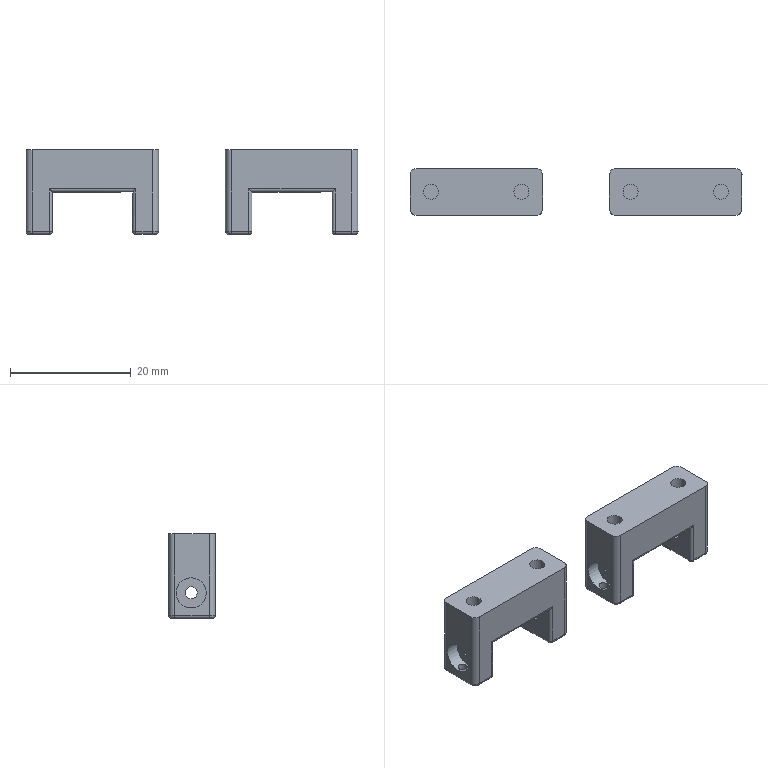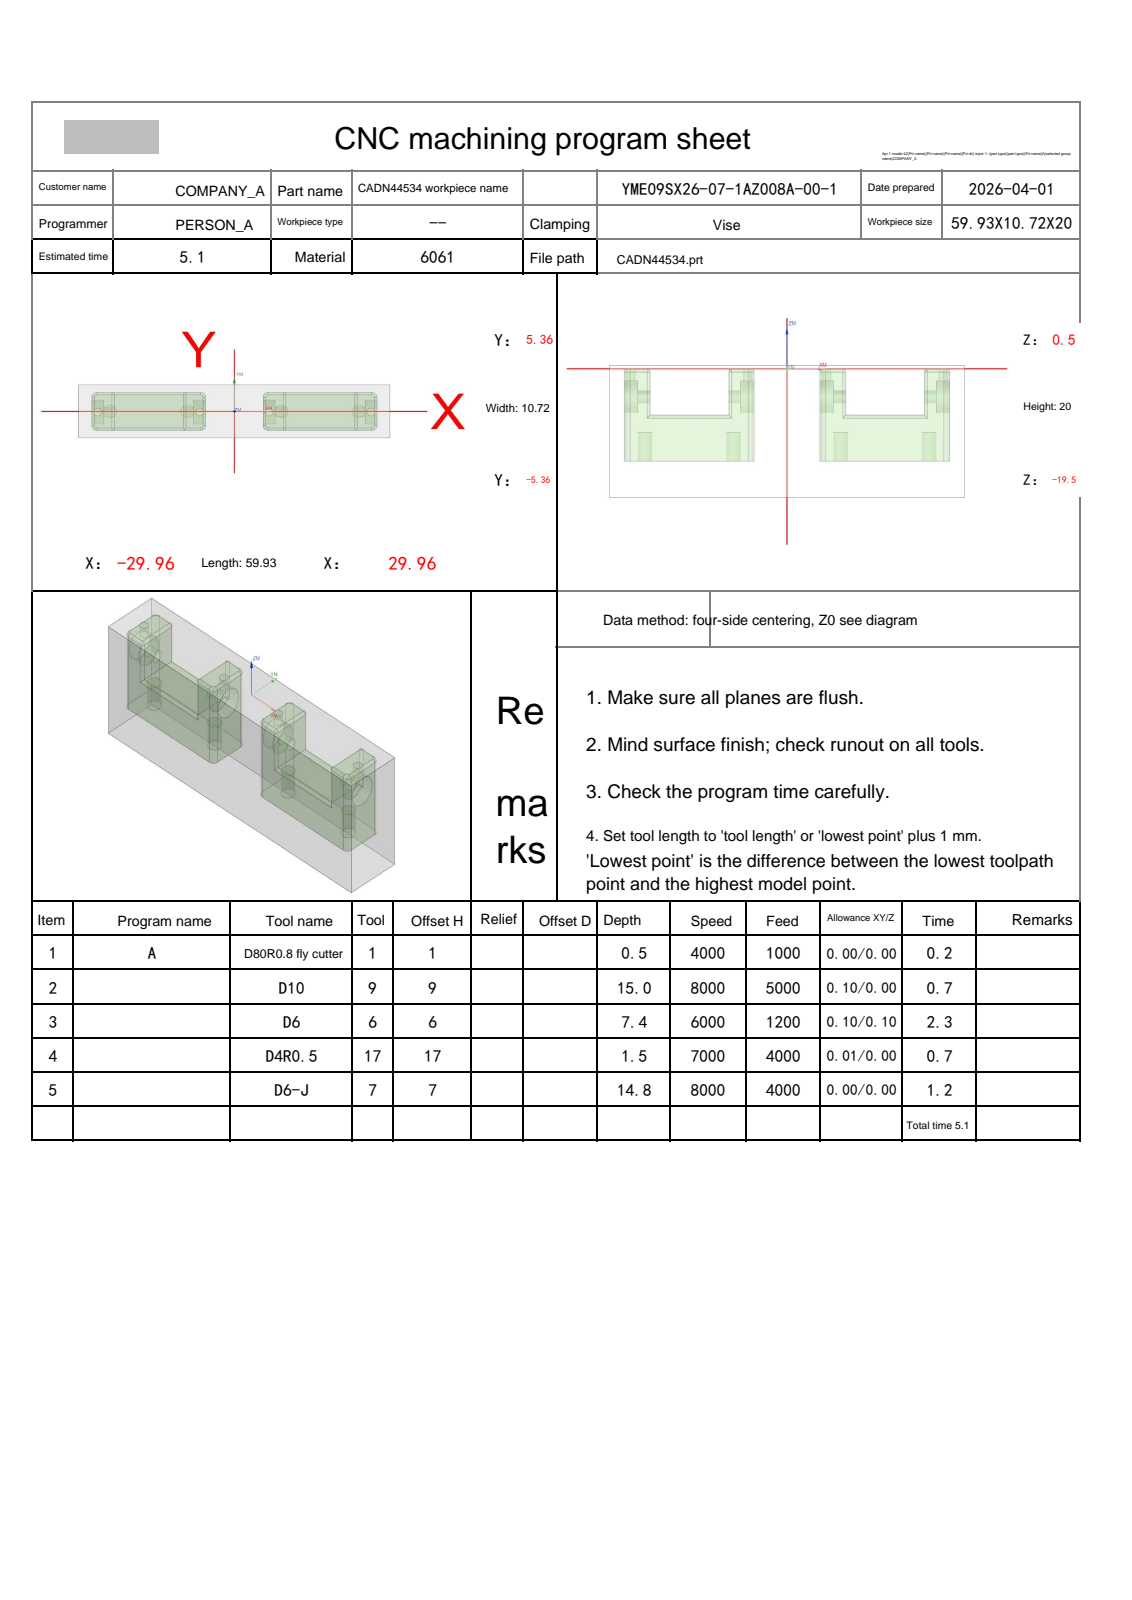NC program | NX | posted by the shop | part box 54.928 x 7.717 x 14 mm
Lines 12390 to 13497 of 13497:
N5 T07 M06
(D6-J  D=6. R=0. H=07 ce=0.30 di=0.00)
G00 G90 G54 X19.883 Y9.358 M03 S6000
G43 H07 Z20.
M08
Z-6.5
G01 Z-7. F1200.
Y6.358
Y-6.358
X16.55
X16.549 Y6.358
X13.216
Y-6.358
Y-9.358
Z-6.5
G00 Z20.
X-13.117 Y9.358
Z-6.5
G01 Z-7.
Y6.358
Y-6.358
X-16.45
X-16.451 Y6.358
X-19.784
Y-6.358
Y-9.358
Z-6.5
G00 Z20.
G00 G90 X-23.417 Y9.866 M03 S7000
Z10.5
Z-6.514
G01 Z-7.014 F4000.
G03 X-23.516 Y9.101 I2.901 J-.765
X-21.928 Y6.455 I3. J0.0
G01 X-21.91
X-21.721 Y6.41
X-21.709 Y6.413
X-11.535 Y6.403
X-11.189 Y6.429
X-10.972 Y6.454
X-10.901 Y6.49 Z-7.018
G02 X-16.443 Y6.429 I-5.541 J250.43
X-21.999 Y6.491 I0.0 J250.491
G01 Z-7.023
X-21.673 Y6.474
G03 X-16.685 Y6.429 I4.987 J272.945
X-10.901 Y6.49 I0.0 J272.991
G01 X-10.817 Y6.532 Z-7.028
X-11.003 Y6.523
X-11.137 Y6.528
X-21.564
X-21.624 Y6.519
X-21.652 Y6.53
X-21.788 Y6.527
X-21.91 Y6.53
X-21.998 Y6.513
X-22.085 Y6.532
X-22.088 Y6.534 Z-7.034
X-21.999 Y6.514
X-21.91 Y6.531
X-21.787 Y6.53
X-21.651 Y6.531
X-21.623 Y6.52
X-21.564 Y6.53
X-10.935 Y6.529
X-10.814 Y6.533
X-10.751 Y6.562 Z-7.039
X-11.151 Y6.553
X-21.607 Y6.547
G02 X-22.146 Y6.561 I1.789 J80.183
G01 X-22.181 Y6.576 Z-7.046
X-22.062 Y6.57
X-21.955 Y6.575
X-21.627 Y6.573
X-21.614 Y6.574
X-21.611 Y6.56
X-21.564 Y6.573
G03 X-16.706 Y6.567 I4.858 J2040.216
X-10.719 Y6.576 I0.0 J2040.222
G01 X-10.686 Y6.59 Z-7.052
G02 X-10.941 Y6.587 I-.256 J8.86
X-11.189 Y6.59 I0.0 J8.864
G01 X-11.535 Y6.589
X-21.564 Y6.59
X-21.578 Y6.571
X-21.602
X-21.617 Y6.589
X-21.785 Y6.583
X-21.959 Y6.59
X-22.083 Y6.582
X-22.213 Y6.59
X-22.246 Y6.604 Z-7.06
X-22.066 Y6.59
X-22.049 Y6.604
X-21.954 Y6.601
X-21.801 Y6.596
X-21.609 Y6.603
X-21.597 Y6.586
X-21.576
X-21.564 Y6.604
X-11.177 Y6.599
X-10.699 Y6.601
X-10.655 Y6.603
X-10.622 Y6.617 Z-7.067
X-10.704 Y6.613
G02 X-16.751 Y6.61 I-6.048 J5802.303
X-21.937 Y6.612 I0.0 J5802.307
G01 X-22.043 Y6.616
X-22.06 Y6.604
X-22.28 Y6.618
X-22.314 Y6.631 Z-7.075
G03 X-22.069 Y6.623 I.244 J3.639
G01 X-21.931 Y6.625
X-19.415
G03 X-11.189 Y6.63 I0.0 J6451.95
G01 X-11.104 Y6.621
G03 X-10.585 Y6.631 I-.883 J59.243
G01 X-10.554 Y6.649 Z-7.083
X-10.576 Y6.643
X-10.714 Y6.638
X-11.189 Y6.642
X-21.669 Y6.64
X-21.724 Y6.634
X-21.911 Y6.643
G02 X-22.127 Y6.637 I-.215 J3.619
X-22.346 Y6.644 I0.0 J3.626
G01 X-22.403 Y6.668 Z-7.092
X-22.361 Y6.647
X-22.314 Y6.653
X-10.843
X-10.52 Y6.662
X-10.486 Y6.671 Z-7.101
X-22.353 Y6.668
X-22.4 Y6.674
X-22.447 Y6.681 Z-7.11
X-10.453 Y6.68
X-10.448 Y6.682
X-10.415 Y6.693 Z-7.12
X-10.454 Y6.689
X-22.441 Y6.69
X-22.49 Y6.694
X-22.522 Y6.705 Z-7.13
X-22.441 Y6.699
X-10.454
X-10.383 Y6.704
X-10.339 Y6.716 Z-7.14
X-10.345 Y6.715
X-10.454 Y6.709
X-22.44
X-22.554 Y6.715
X-22.596 Y6.727 Z-7.151
X-22.44 Y6.719
X-10.444 Y6.72
X-10.378 Y6.722
X-10.307 Y6.727
X-10.275 Y6.736 Z-7.162
X-10.378 Y6.731
X-22.439 Y6.73
X-22.629 Y6.737
X-22.662 Y6.747 Z-7.173
X-22.514 Y6.741
X-10.379
X-10.232 Y6.748
X-10.2 Y6.756 Z-7.185
X-10.379 Y6.751
X-17.068 Y6.75
X-22.557 Y6.751
X-22.705 Y6.757
X-22.738 Y6.766 Z-7.197
X-22.634 Y6.762
X-10.303 Y6.761
X-10.195 Y6.764
X-10.157 Y6.767
X-10.124 Y6.775 Z-7.209
X-22.77 Y6.774
X-22.813 Y6.783 Z-7.221
X-22.743 Y6.78
X-10.347
X-10.092 Y6.783
X-10.049 Y6.792 Z-7.234
X-10.239 Y6.788
X-22.818 Y6.79
X-22.845 Y6.791
X-22.888 Y6.8 Z-7.247
X-22.818 Y6.797
X-10.016 Y6.799
X-9.973 Y6.807 Z-7.26
X-22.926 Y6.806
X-22.931 Y6.807
X-22.964 Y6.814 Z-7.273
X-9.941 Y6.813
X-9.898 Y6.821 Z-7.287
X-23.007
X-23.039 Y6.826 Z-7.3
X-9.854 Y6.827
X-9.822 Y6.832 Z-7.314
X-23.083 Y6.833
X-23.115 Y6.838 Z-7.328
X-9.779
X-9.746 Y6.843 Z-7.342
X-23.158
X-23.191 Y6.847 Z-7.357
X-9.703 Y6.848
X-9.66 Y6.852 Z-7.371
X-9.698 Y6.85
X-10.23 Y6.851
X-22.433 Y6.848
X-22.502
G02 X-23.234 Y6.851 I0.0 J80.325
G01 X-23.266 Y6.855 Z-7.386
G03 X-22.664 Y6.848 I1.661 J130.188
G01 X-22.653 Y6.854
X-22.443 Y6.851
G03 X-16.454 Y6.839 I5.99 J1587.495
X-9.655 Y6.854 I0.0 J1587.507
G01 X-9.628 Y6.855
X-9.584 Y6.859 Z-7.401
X-9.655 Y6.856
X-22.443 Y6.853
X-22.66 Y6.852
G02 X-23.31 Y6.858 I0.0 J35.767
G01 X-23.354 Y6.861 Z-7.415
G03 X-22.679 Y6.855 I.674 J34.304
G01 X-22.443
X-9.785 Y6.858
X-9.774 Y6.854
X-9.552 Y6.861
X-9.52 Y6.863 Z-7.43
X-9.59 Y6.861
X-23.12 Y6.856
X-23.376 Y6.863
X-23.418 Y6.865 Z-7.445
X-23.12 Y6.859
X-9.525 Y6.864
X-9.487 Y6.865
G00 Z-6.96
X-4.77 Y9.642
G01 Z-7.46
G02 X-7.758 Y6.868 I-2.991 J.226
G01 X-9.46 Y6.866
X-23.445
X-25.147 Y6.868
X-25.179 Z-7.475
X-23.293 Y6.866
X-9.46 Y6.867
X-7.726 Y6.868
X-7.693 Z-7.49
X-25.211
X-25.239 Z-7.5
X-7.666
G00 Z10.5
X-9.5 Y-9.862
Z-6.514
G01 Z-7.014
G03 X-9.4 Y-9.092 I-2.9 J.77
X-10.972 Y-6.454 I-3. J0.0
G01 X-11.535 Y-6.403
X-21.564
X-21.722 Y-6.41
X-21.91 Y-6.454
X-21.931 Y-6.455
X-21.999 Y-6.49 Z-7.018
G02 X-16.428 Y-6.428 I5.57 J-250.081
X-10.903 Y-6.489 I0.0 J-250.143
G01 Z-7.023
X-21.674 Y-6.473
X-21.826 Y-6.47
X-21.999 Y-6.49
X-22.085 Y-6.533 Z-7.028
X-21.967 Y-6.527
X-21.95 Y-6.519
X-21.901 Y-6.544
X-21.845 Y-6.545
X-21.795 Y-6.523
X-21.719 Y-6.541
X-21.642 Y-6.528
X-21.635 Y-6.521
X-21.564 Y-6.528
X-11.136 Y-6.527
X-11.093 Y-6.525
X-10.999 Y-6.522
X-10.815 Y-6.532
X-10.813 Y-6.534 Z-7.034
G03 X-11.04 Y-6.524 I-.228 J-2.737
G01 X-11.168 Y-6.527
X-11.189 Y-6.531
X-21.564 Y-6.53
X-21.624 Y-6.52
X-21.633 Y-6.538
X-21.652 Y-6.531
X-21.757 Y-6.529
X-21.91 Y-6.533
X-21.924 Y-6.513
X-21.949 Y-6.511
X-21.966 Y-6.529
X-21.978 Y-6.527
X-22.088 Y-6.534
X-22.149 Y-6.562 Z-7.039
X-21.963 Y-6.558
X-21.935 Y-6.55
G02 X-17.545 Y-6.542 I4.39 J-1137.616
X-10.753 Y-6.562 I0.0 J-1137.625
G01 X-10.719 Y-6.576 Z-7.046
X-11.182 Y-6.573
X-21.564
X-21.582 Y-6.555
X-21.609 Y-6.554
X-21.627 Y-6.573
X-21.808 Y-6.572
G03 X-22.182 Y-6.577 I0.0 J-13.564
G01 X-22.215 Y-6.591 Z-7.052
X-22.176 Y-6.587
X-21.959 Y-6.59
X-21.778 Y-6.583
X-21.606 Y-6.589
X-21.597 Y-6.569
X-21.573
X-21.564 Y-6.59
X-10.827 Y-6.585
X-10.689 Y-6.59
X-10.658 Y-6.603 Z-7.06
G03 X-10.926 Y-6.598 I-.269 J-7.167
X-11.189 Y-6.603 I0.0 J-7.172
G01 X-11.535 Y-6.601
X-21.218 Y-6.602
X-21.564 Y-6.604
X-21.576 Y-6.586
X-21.597
X-21.61 Y-6.603
G03 X-21.822 Y-6.597 I-.212 J-3.885
X-22.049 Y-6.604 I0.0 J-3.89
G01 X-22.148 Y-6.587
X-22.247 Y-6.604
X-22.282 Y-6.618 Z-7.067
X-22.161 Y-6.611
X-22.055 Y-6.616
G02 X-21.807 Y-6.611 I.247 J-5.936
X-21.603 Y-6.615 I0.0 J-5.941
G01 X-21.592 Y-6.613
X-10.964 Y-6.612
X-10.879
G02 X-10.621 Y-6.618 I0.0 J-5.401
G01 X-10.588 Y-6.631 Z-7.075
G03 X-10.894 Y-6.625 I-.306 J-7.786
X-11.189 Y-6.63 I0.0 J-7.792
X-18.245 Y-6.624 I-7.055 J-3932.721
X-22.194 Y-6.626 I0.0 J-3932.727
G01 X-22.312 Y-6.631
X-22.349 Y-6.644 Z-7.083
X-22.256 Y-6.641
G02 X-14.927 Y-6.637 I7.328 J-6094.405
X-10.978 Y-6.638 I0.0 J-6094.409
G01 X-10.637 Y-6.642
X-10.553 Y-6.649
X-10.517 Y-6.661 Z-7.092
X-10.582 Y-6.655
X-11.189 Y-6.654
X-21.673
X-22.326
X-22.367 Y-6.648
X-22.403 Y-6.668
X-22.4 Y-6.674 Z-7.101
X-22.353 Y-6.668
X-10.498 Y-6.669
X-10.482 Y-6.672
X-10.445 Y-6.682 Z-7.11
X-22.446 Y-6.681
X-22.478 Y-6.691 Z-7.12
X-22.451 Y-6.69
X-10.453
X-10.409 Y-6.694
X-10.377 Y-6.705 Z-7.13
X-10.454 Y-6.699
X-22.451
X-22.521 Y-6.704
X-22.553 Y-6.715 Z-7.14
X-22.483 Y-6.71
X-22.451 Y-6.709
X-10.456
X-10.344 Y-6.715
X-10.312 Y-6.726 Z-7.151
X-10.458 Y-6.719
X-22.45
X-22.483 Y-6.72
X-22.591 Y-6.725
X-22.596 Y-6.727
X-22.629 Y-6.736 Z-7.162
X-22.623 Y-6.735
X-22.515 Y-6.73
X-10.447 Y-6.729
X-10.271 Y-6.737
X-10.24 Y-6.747 Z-7.173
X-10.449 Y-6.739
X-22.515 Y-6.74
X-22.662 Y-6.746
X-22.694 Y-6.755 Z-7.185
X-10.451 Y-6.75
X-10.198 Y-6.757
X-10.168 Y-6.765 Z-7.197
X-10.216 Y-6.763
X-22.689 Y-6.762
X-22.737 Y-6.766
X-22.77 Y-6.774 Z-7.209
X-10.134 Y-6.773
X-10.089 Y-6.783 Z-7.221
X-22.813
X-22.845 Y-6.791 Z-7.234
X-22.622 Y-6.789
X-10.221 Y-6.788
X-10.045 Y-6.792
X-10.002 Y-6.8 Z-7.247
X-10.007 Y-6.799
X-22.888 Y-6.8
X-22.92 Y-6.806 Z-7.26
X-22.698 Y-6.804
X-10.052
X-9.981 Y-6.806
X-9.938 Y-6.813 Z-7.273
X-10.171 Y-6.812
X-22.523 Y-6.811
X-22.953 Y-6.813
X-22.996 Y-6.82 Z-7.287
X-9.907 Y-6.819
X-9.864 Y-6.826 Z-7.3
X-10.173 Y-6.824
X-23.039 Y-6.826
X-23.083 Y-6.833 Z-7.314
X-9.903 Y-6.83
X-9.822 Y-6.832
X-9.79 Y-6.837 Z-7.328
X-9.828
X-23.115
X-23.147 Y-6.842 Z-7.342
X-9.746
X-9.714 Y-6.847 Z-7.357
X-23.191
X-23.234 Y-6.851 Z-7.371
G02 X-16.452 Y-6.835 I6.782 J-1442.526
X-9.671 Y-6.851 I0.0 J-1442.542
G01 X-9.638 Y-6.854 Z-7.386
G03 X-16.44 Y-6.836 I-6.802 J-1254.871
X-23.266 Y-6.855 I0.0 J-1254.89
G01 X-23.299 Y-6.857 Z-7.401
X-23.142 Y-6.851
X-23.12 Y-6.856
G02 X-16.506 Y-6.839 I6.614 J-1278.773
X-9.595 Y-6.857 I0.0 J-1278.79
G01 X-9.552 Y-6.86 Z-7.415
X-9.665 Y-6.857
X-23.239
X-23.304 Y-6.859
X-23.342 Y-6.86
X-23.385 Y-6.863 Z-7.43
X-22.925 Y-6.86
X-9.557 Y-6.861
X-9.509 Y-6.863
G00 Z-6.945
X-4.774 Y-9.643
G01 Z-7.445
G03 X-7.758 Y-6.868 I-2.992 J-.225
G01 X-9.514 Y-6.864
X-23.347 Y-6.863
X-25.147 Y-6.868
X-25.168 Z-7.46
X-23.444 Y-6.866
X-9.503
X-7.736 Y-6.868
X-7.704 Z-7.475
X-9.514 Y-6.866
X-23.39 Y-6.867
X-25.19 Y-6.868
X-25.222 Z-7.49
X-7.683
X-7.656 Z-7.5
X-25.239
G00 Z10.5
X9.591 Y9.864
Z-6.514
G01 Z-7.014
G03 X9.492 Y9.097 I2.9 J-.767
X11.072 Y6.454 I3. J0.0
G01 X11.635 Y6.403
X21.664
X21.821 Y6.41
X22.01 Y6.454
X22.03
X22.099 Y6.49 Z-7.018
G02 X16.546 Y6.429 I-5.553 J250.316
X11.001 Y6.49 I0.0 J250.377
G01 Z-7.023
G03 X16.77 Y6.429 I5.769 J270.899
X21.771 Y6.475 I0.0 J270.96
G01 X22.099 Y6.49
X22.184 Y6.532 Z-7.028
X22.116 Y6.541
X22.051 Y6.519
X22.01 Y6.53
X21.751
X21.723 Y6.518
X21.664 Y6.528
X11.236
X11.193 Y6.525
X11.095 Y6.522
X10.916 Y6.532
X10.913 Y6.534 Z-7.034
X11.092 Y6.524
X11.177 Y6.526
X11.237 Y6.529
X21.664
X21.722 Y6.52
X21.75 Y6.531
X22.01
X22.051 Y6.52
X22.117 Y6.542
X22.186 Y6.533
X22.246 Y6.561 Z-7.039
G02 X21.706 Y6.547 I-2.672 J92.571
G01 X21.664 Y6.556
X11.276 Y6.557
X10.854 Y6.561
X10.822 Y6.575 Z-7.046
X11.286 Y6.574
X21.664 Y6.572
X21.71 Y6.561
X21.713 Y6.575
X21.884 Y6.568
X22.055 Y6.576
X22.168 Y6.57
X22.28 Y6.575
X22.315 Y6.59 Z-7.052
X22.153 Y6.582
X22.01 Y6.589
X21.859 Y6.578
X21.705 Y6.589
X21.701 Y6.576
X21.664 Y6.589
X11.289 Y6.591
G02 X11.032 Y6.586 I-.257 J7.365
X10.787 Y6.59 I0.0 J7.369
G01 X10.753 Y6.604 Z-7.06
G03 X11.018 Y6.598 I.265 J6.214
X11.289 Y6.604 I0.0 J6.22
G01 X21.318 Y6.602
X21.664 Y6.603
X21.692 Y6.592
X21.724 Y6.619
X21.766 Y6.618
X21.797 Y6.59
X22.15 Y6.603
Y6.588
X22.165 Y6.591
X22.344 Y6.603
X22.379 Y6.617 Z-7.067
X22.159 Y6.604
X22.145 Y6.601
X22.144 Y6.615
X21.789 Y6.603
X21.762 Y6.629
X21.723 Y6.634
X21.69 Y6.614
X21.664 Y6.618
X11.285 Y6.616
X11.197 Y6.608
G02 X10.72 Y6.618 I2.061 J116.415
G01 X10.686 Y6.631 Z-7.075
G03 X10.992 Y6.624 I.306 J6.604
X11.289 Y6.631 I0.0 J6.611
G01 X11.635 Y6.626
X21.682 Y6.628
X21.836 Y6.621
X22.01 Y6.63
X22.203 Y6.623
G03 X22.413 Y6.631 I0.0 J2.68
G01 X22.447 Y6.644 Z-7.083
X22.288 Y6.638
G02 X18.088 Y6.637 I-4.2 J5603.073
X10.943 Y6.641 I0.0 J5603.074
G01 X10.894 Y6.635
X10.676 Y6.643
X10.654 Y6.649
X10.619 Y6.662 Z-7.092
X10.943 Y6.654
X21.749 Y6.653
X22.427 Y6.654
X22.467 Y6.648
X22.503 Y6.668
X22.5 Y6.674 Z-7.101
X22.39 Y6.667
X10.585 Y6.672
X10.547 Y6.682 Z-7.11
X22.546 Y6.681
X22.589 Y6.694 Z-7.12
X22.541 Y6.689
X10.553 Y6.69
X10.514 Y6.693
X10.482 Y6.704 Z-7.13
X10.554 Y6.699
X22.551
X22.621 Y6.705
X22.653 Y6.715 Z-7.14
X22.551 Y6.709
X10.554
X10.444 Y6.715
X10.439 Y6.717
X10.406 Y6.727 Z-7.151
X10.555 Y6.719
X22.55
X22.615 Y6.721
X22.696 Y6.727
X22.729 Y6.737 Z-7.162
X22.615 Y6.731
X10.555 Y6.73
X10.375 Y6.736
X10.332 Y6.747 Z-7.173
X10.445 Y6.742
X22.614 Y6.741
X22.762 Y6.747
X22.805 Y6.757 Z-7.185
X22.734 Y6.753
X22.647 Y6.751
X10.446
X10.3 Y6.756
X10.258 Y6.766 Z-7.197
X10.37 Y6.762
X15.785 Y6.761
X22.614
X22.837 Y6.766
X22.881 Y6.776 Z-7.209
X22.875 Y6.775
X10.225
X10.192 Y6.783 Z-7.221
X10.263 Y6.78
X22.645 Y6.781
X22.913 Y6.783
X22.945 Y6.791 Z-7.234
X10.149 Y6.792
X10.116 Y6.799 Z-7.247
X10.154 Y6.798
X22.988 Y6.8
X23.031 Y6.807 Z-7.26
X10.154 Y6.804
X10.073 Y6.807
X10.041 Y6.813 Z-7.273
X23.064 Y6.814
X23.107 Y6.821 Z-7.287
X9.998
X9.954 Y6.827 Z-7.3
X9.96 Y6.826
X22.798 Y6.825
X23.139 Y6.826
X23.183 Y6.833 Z-7.314
X23.134 Y6.831
X9.922 Y6.832
X9.879 Y6.838 Z-7.328
X23.215
X23.247 Y6.842 Z-7.342
X9.846 Y6.843
X9.803 Y6.848 Z-7.357
X22.356 Y6.846
X22.515
G03 X23.291 Y6.847 I0.0 J213.431
G01 X23.334 Y6.851 Z-7.371
G02 X16.493 Y6.838 I-6.84 J1774.339
X10.561 Y6.848 I0.0 J1774.352
G01 X10.441
G02 X9.76 Y6.852 I0.0 J58.753
G01 X9.728 Y6.855 Z-7.386
X9.862 Y6.853
G03 X16.455 Y6.839 I6.593 J1568.063
X23.366 Y6.855 I0.0 J1568.077
G01 X23.41 Y6.858 Z-7.401
X23.242 Y6.852
X23.22 Y6.856
X10.562 Y6.853
X10.352 Y6.852
G02 X9.684 Y6.859 I0.0 J35.275
G01 X9.652 Y6.861 Z-7.415
G03 X10.315 Y6.855 I.663 J33.373
G01 X10.551
X23.22 Y6.858
X23.242 Y6.854
X23.454 Y6.861
X23.476 Y6.863 Z-7.43
X23.393 Y6.861
X9.733 Y6.86
X9.62 Y6.863
X9.587 Y6.865 Z-7.445
X9.874 Y6.859
X23.242 Y6.86
X23.518 Y6.865
G00 Z-6.96
X28.236 Y9.641
G01 Z-7.46
G02 X25.247 Y6.868 I-2.991 J.227
G01 X23.555 Y6.867
X9.56 Y6.866
X7.858 Y6.868
X7.826 Z-7.475
X9.874 Y6.865
X22.764 Y6.866
X25.279 Y6.868
X25.311 Z-7.49
X7.793
X7.766 Z-7.5
X25.339
G00 Z10.5
X23.505 Y-9.863
Z-6.514
G01 Z-7.014
G03 X23.605 Y-9.095 I-2.9 J.768
X22.029 Y-6.454 I-3. J0.0
G01 X22.01 Y-6.453
X21.814 Y-6.409
X11.635 Y-6.403
X11.289 Y-6.431
X11.072 Y-6.454
X11.002 Y-6.49 Z-7.018
G02 X16.546 Y-6.428 I5.543 J-249.45
X22.099 Y-6.49 I0.0 J-249.512
G01 Z-7.023
G03 X16.546 Y-6.428 I-5.553 J-249.45
X11.002 Y-6.49 I0.0 J-249.512
G01 X10.914 Y-6.533 Z-7.028
X11.108 Y-6.522
X11.237 Y-6.527
X21.664 Y-6.528
X21.729 Y-6.519
X21.739 Y-6.543
X21.764 Y-6.537
X21.916 Y-6.525
X22.01 Y-6.53
X22.067 Y-6.512
X22.128 Y-6.513
X22.185 Y-6.532
X22.187 Y-6.533 Z-7.034
X22.129 Y-6.514
X22.068 Y-6.513
X22.01 Y-6.531
X21.916 Y-6.528
X21.754 Y-6.539
X21.732 Y-6.543
X21.728 Y-6.52
X21.664 Y-6.529
X11.635 Y-6.53
X11.289 Y-6.531
X11.268 Y-6.527
X11.14 Y-6.524
G03 X10.911 Y-6.534 I0.0 J-2.635
G01 X10.851 Y-6.562 Z-7.039
X11.252 Y-6.553
X21.714 Y-6.546
X21.802 Y-6.553
X21.891 Y-6.552
G02 X22.248 Y-6.562 I0.0 J-6.403
G01 X22.281 Y-6.577 Z-7.046
X22.16 Y-6.568
X22.058 Y-6.574
X21.872 Y-6.568
X21.722 Y-6.572
X21.708 Y-6.576
X21.705 Y-6.561
X21.664 Y-6.572
X11.282 Y-6.574
X10.818 Y-6.577
X10.786 Y-6.591 Z-7.052
G02 X11.032 Y-6.586 I.246 J-7.507
X11.289 Y-6.591 I0.0 J-7.511
G01 X12.673 Y-6.59
X19.935 Y-6.586
X21.664 Y-6.588
X21.696 Y-6.577
X21.701 Y-6.588
X21.853 Y-6.577
X22.01 Y-6.589
X22.155 Y-6.582
X22.31 Y-6.59
X22.345 Y-6.603 Z-7.06
X22.152 Y-6.59
X22.133 Y-6.584
X22.128 Y-6.603
X21.781 Y-6.589
X21.779 Y-6.606
X21.764 Y-6.6
X11.277
X10.827 Y-6.599
X10.753 Y-6.604
X10.719 Y-6.618 Z-7.067
X10.801 Y-6.613
X13. Y-6.614
G03 X15.785 Y-6.613 I0.0 J2481.023
G01 X21.699
X21.755 Y-6.615
X21.76 Y-6.595
X21.778 Y-6.601
X22.01 Y-6.618
X22.194 Y-6.608
X22.379 Y-6.618
X22.413 Y-6.631 Z-7.075
G03 X22.209 Y-6.622 I-.204 J-2.299
G01 X22.01 Y-6.63
X21.77 Y-6.615
X21.753 Y-6.609
X21.749 Y-6.627
X21.691 Y-6.626
X11.057
G03 X10.687 Y-6.631 I.001 J-15.968
G01 X10.654 Y-6.649 Z-7.083
X10.677 Y-6.643
X10.943 Y-6.641
G02 X16.644 Y-6.632 I5.701 J-1662.594
X21.741 Y-6.639 I0.0 J-1662.604
G01 X21.757 Y-6.632
X21.835 Y-6.634
G03 X22.447 Y-6.644 I2.221 J120.346
G01 X22.505 Y-6.668 Z-7.092
X22.459 Y-6.656
X22.128 Y-6.648
X22.105 Y-6.653
X21.734
X10.943 Y-6.654
X10.62 Y-6.662
X10.586 Y-6.671 Z-7.101
X10.598 Y-6.668
X22.455
X22.502 Y-6.674
X22.553 Y-6.681 Z-7.11
X10.548 Y-6.682
X10.515 Y-6.693 Z-7.12
X10.554 Y-6.69
X22.546
X22.583 Y-6.692
X22.624 Y-6.705 Z-7.13
X22.544 Y-6.699
X10.554
X10.483 Y-6.704
X10.44 Y-6.716 Z-7.14
X10.521 Y-6.71
X10.554 Y-6.709
X22.542
X22.655 Y-6.715
X22.696 Y-6.727 Z-7.151
X22.54 Y-6.719
X10.544
X10.407 Y-6.726
X10.375 Y-6.736 Z-7.162
X10.489 Y-6.73
X10.544 Y-6.729
X22.538
X22.731 Y-6.737
X22.765 Y-6.747 Z-7.173
X22.623 Y-6.74
X10.343 Y-6.745
X10.3 Y-6.756 Z-7.185
X10.37 Y-6.752
X18.897 Y-6.748
X22.643 Y-6.75
X22.798 Y-6.757
X22.841 Y-6.766 Z-7.197
X22.641 Y-6.76
X18.897 Y-6.758
X10.523 Y-6.761
X10.306 Y-6.763
X10.257 Y-6.767
X10.225 Y-6.775 Z-7.209
X22.868 Y-6.773
X22.874 Y-6.774
X22.905 Y-6.782 Z-7.221
X22.789 Y-6.779
X10.382 Y-6.78
X10.192 Y-6.783
X10.149 Y-6.792 Z-7.234
X22.947 Y-6.791
X22.989 Y-6.799 Z-7.247
X22.752 Y-6.797
X10.546 Y-6.796
X10.116 Y-6.799
X10.073 Y-6.807 Z-7.26
X10.296 Y-6.804
X22.897 Y-6.803
X23.021 Y-6.806
X23.064 Y-6.813 Z-7.273
X10.041
X10.008 Y-6.819 Z-7.287
X23.097 Y-6.82
X23.141 Y-6.826 Z-7.3
X9.96
X9.954 Y-6.827
X9.922 Y-6.832 Z-7.314
X23.173
X23.205 Y-6.837 Z-7.328
X9.884 Y-6.838
X9.854 Y-6.842 Z-7.342
X10.068 Y-6.841
X23.248 Y-6.842
X23.291 Y-6.847 Z-7.357
X9.809
X9.765 Y-6.851 Z-7.371
G02 X16.55 Y-6.836 I6.785 J-1467.914
X23.334 Y-6.851 I0.0 J-1467.93
G01 X23.366 Y-6.854 Z-7.386
G03 X16.551 Y-6.837 I-6.815 J-1344.293
X9.735 Y-6.854 I0.0 J-1344.311
G01 X9.691 Y-6.858 Z-7.401
X9.862 Y-6.851
X9.877 Y-6.856
X23.242 Y-6.852
X23.399 Y-6.857
X23.442 Y-6.86 Z-7.415
X23.339 Y-6.857
X9.758
X9.661 Y-6.86
X9.615 Y-6.863 Z-7.43
X9.683 Y-6.861
X23.436
X23.496 Y-6.863
G00 Z-6.945
X28.22 Y-9.645
G01 Z-7.445
G03 X25.236 Y-6.868 I-2.992 J-.223
G01 X23.49 Y-6.864
X9.669 Y-6.863
X7.858 Y-6.868
X7.836 Z-7.46
X9.56 Y-6.866
X23.501
X25.268 Y-6.868
X25.29 Z-7.475
X23.393 Y-6.866
X9.56 Y-6.867
X7.804 Y-6.868
X7.783 Z-7.49
X25.322
X25.339 Z-7.5
X7.756
G00 Z10.5
G00 G90 X9.668 Y7.951 M03 S8000
Z5.5
Z-6.15
G01 Z-7.15 F1000.
G41 D07
Y7.61
G03 X10.568 Y6.71 I.9 J0.0
G01 X22.502 Y6.707
X22.678 Y6.714
G02 X23.684 Y6.858 I1.018 J-3.532
G01 X26.464
G02 X30.464 Y2.858 I0.0 J-4.
G01 Y-2.858
G02 X26.464 Y-6.858 I-4. J0.0
G01 X23.684
G02 X22.679 Y-6.714 I.023 J3.737
G01 X22.502 Y-6.707
X10.471 Y-6.711
X10.386 Y-6.722
X10.147 Y-6.778
G02 X9.446 Y-6.858 I-.7 J3.
G01 X6.536
G02 X2.536 Y-2.858 I0.0 J4.
G01 Y2.858
G02 X6.536 Y6.858 I4. J0.0
G01 X9.416
G02 X10.311 Y6.743 I-.002 J-3.533
G03 X10.568 Y6.71 I.258 J.983
X11.468 Y7.609 I0.0 J.9
G01 G40 Y7.809
Z-6.15
G00 Z5.5
X-23.387 Y7.953
Z-6.15
G01 Z-7.15
G41 D07
X-23.416 Y7.755
X-23.425 Y7.626
G03 X-22.676 Y6.739 I.9 J0.0
G01 X-22.502 Y6.709
X-22.156 Y6.713
X-10.386 Y6.71
X-10.298 Y6.719
G02 X-9.316 Y6.858 I.982 J-3.381
G01 X-6.536
G02 X-2.536 Y2.858 I0.0 J-4.
G01 Y-2.858
G02 X-6.536 Y-6.858 I-4. J0.0
G01 X-9.316
G02 X-10.297 Y-6.717 I.006 J3.527
G01 X-10.386 Y-6.71
X-22.503 Y-6.713
X-22.583 Y-6.709
X-22.659 Y-6.734
G02 X-23.582 Y-6.858 I-.923 J3.375
G01 X-23.584
X-26.464
G02 X-30.464 Y-2.858 I0.0 J4.
G01 Y2.858
G02 X-26.464 Y6.858 I4. J0.0
G01 X-23.584
X-23.582
G02 X-22.676 Y6.739 I0.0 J-3.501
G03 X-22.443 Y6.708 I.233 J.869
X-21.573 Y7.375 I0.0 J.9
G01 X-21.51 Y7.613
G40 X-21.458 Y7.806
Z-6.15
G00 Z5.5
X-10.853 Y-7.693
Z-6.
G01 Z-7.
G41 D07
X-10.768 Y-7.512
G03 X-10.683 Y-7.13 I-.815 J.382
X-11.119 Y-6.358 I-.9 J0.0
G02 X-12.816 Y-3.358 I1.803 J3.
G01 Y3.358
G02 X-11.119 Y6.358 I3.5 J0.0
G03 X-10.683 Y7.13 I-.464 J.771
X-10.768 Y7.512 I-.9 J0.0
G01 G40 X-10.853 Y7.693
Z-6.
G00 Z5.5
X22.147 Y-7.693
Z-6.
G01 Z-7.
G41 D07
X22.232 Y-7.512
G03 X22.318 Y-7.13 I-.815 J.382
X21.881 Y-6.358 I-.9 J0.0
G02 X20.184 Y-3.432 I1.803 J3.001
G01 Y-3.089
Y3.358
G02 X21.881 Y6.358 I3.5 J0.0
G03 X22.317 Y7.13 I-.464 J.771
X22.232 Y7.512 I-.9 J0.0
G01 G40 X22.147 Y7.693
Z-6.
G00 Z5.5
X10.953
Z-6.
G01 Z-7.
G41 D07
X10.868 Y7.512
G03 X10.783 Y7.13 I.815 J-.382
X11.219 Y6.358 I.9 J0.0
G02 X12.916 Y3.358 I-1.803 J-3.
G01 Y-3.361
G02 X12.603 Y-4.805 I-3.489 J0.0
X11.22 Y-6.358 I-3.186 J1.446
G03 X10.783 Y-7.13 I.464 J-.771
X10.868 Y-7.512 I.9 J0.0
G01 G40 X10.953 Y-7.693
Z-6.
G00 Z5.5
X-22.047 Y7.693
Z-6.
G01 Z-7.
G41 D07
X-22.132 Y7.512
G03 X-22.217 Y7.13 I.815 J-.382
X-21.781 Y6.358 I.9 J0.0
G02 X-20.084 Y3.358 I-1.803 J-3.
G01 Y-3.358
G02 X-21.781 Y-6.358 I-3.5 J0.0
G03 X-22.217 Y-7.13 I.464 J-.771
X-22.132 Y-7.512 I.9 J0.0
G01 G40 X-22.047 Y-7.693
Z-6.
G00 Z5.5
X-5.622 Y-7.875
Z-13.3
G01 Z-14.3
G41 D07
X-5.64 Y-7.676
G03 X-6.536 Y-6.858 I-.896 J-.083
G01 X-26.464
G02 X-30.464 Y-2.858 I0.0 J4.
G01 Y2.858
G02 X-26.463 Y6.858 I4.001 J-.001
G01 X-6.536
G02 X-2.536 Y2.858 I0.0 J-4.
G01 Y-2.858
G02 X-6.536 Y-6.858 I-4. J0.0
G03 X-7.436 Y-7.758 I0.0 J-.9
G01 G40 Y-7.958
Z-13.3
G00 Z5.5
X27.378 Y-7.875
Z-13.3
G01 Z-14.3
G41 D07
X27.36 Y-7.676
G03 X26.464 Y-6.858 I-.896 J-.083
G01 X6.536
G02 X2.536 Y-2.858 I0.0 J4.
G01 Y2.858
G02 X6.536 Y6.858 I4. J0.0
G01 X26.462
G02 X30.464 Y2.858 I0.0 J-4.001
G01 Y-2.858
G02 X26.464 Y-6.858 I-4. J0.0
G03 X25.564 Y-7.758 I0.0 J-.9
G01 G40 Y-7.958
Z-13.3
G00 Z5.5
M05
M09
G91 G28 Z0.0
G91 G28 Y0.0
M30
%